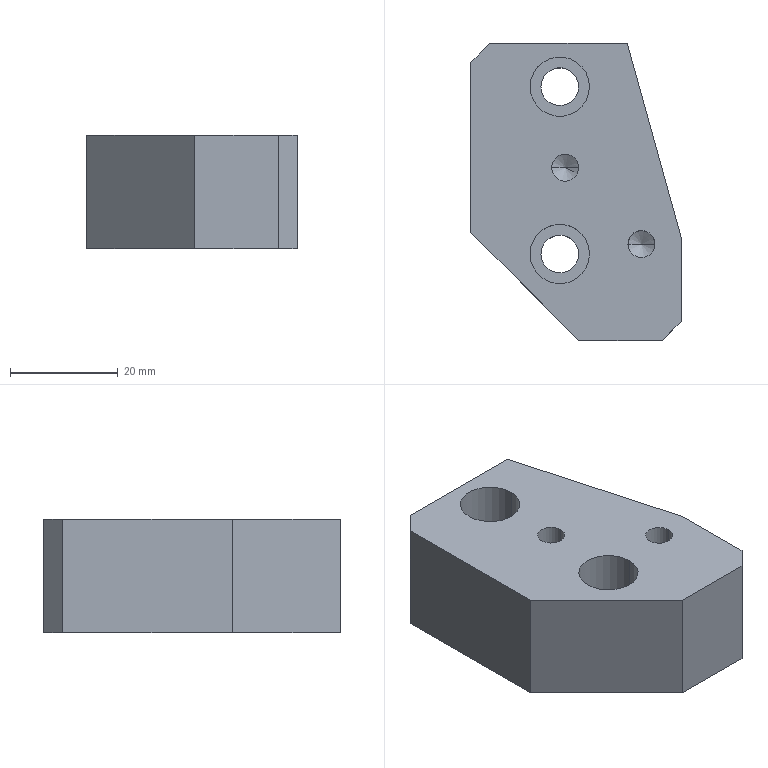Part | SolidWorks | features ICE 2, 3DProfileFeature 1, Extrusion 1, HoleWzd 1 | 1 solid | 28 faces | box 39 x 55 x 21 mm | volume 33486 mm3 | cylinder 12 | plane 12 | cone 4 | commonest cylinder face diameters 5 x4 7 x4 11 x4
STEP:
#1=CARTESIAN_POINT('',(15.,32.,4.));
#2=VERTEX_POINT('',#1);
#3=CARTESIAN_POINT('',(20.,32.,4.));
#4=VERTEX_POINT('',#3);
#5=CARTESIAN_POINT('',(17.5,32.,4.));
#6=DIRECTION('',(0.,0.,1.));
#7=DIRECTION('',(1.,0.,0.));
#8=AXIS2_PLACEMENT_3D('',#5,#6,#7);
#9=CIRCLE('',#8,2.5);
#10=EDGE_CURVE('',#2,#4,#9,.T.);
#11=ORIENTED_EDGE('',*,*,#10,.F.);
#12=CARTESIAN_POINT('',(15.,32.,21.));
#13=VERTEX_POINT('',#12);
#14=CARTESIAN_POINT('',(15.,32.,21.));
#15=DIRECTION('',(0.,0.,1.));
#16=VECTOR('',#15,1000.);
#17=LINE('',#14,#16);
#18=EDGE_CURVE('',#2,#13,#17,.T.);
#19=ORIENTED_EDGE('',*,*,#18,.T.);
#20=CARTESIAN_POINT('',(20.,32.,21.));
#21=VERTEX_POINT('',#20);
#22=CARTESIAN_POINT('',(17.5,32.,21.));
#23=DIRECTION('',(0.,0.,1.));
#24=DIRECTION('',(1.,0.,0.));
#25=AXIS2_PLACEMENT_3D('',#22,#23,#24);
#26=CIRCLE('',#25,2.5);
#27=EDGE_CURVE('',#13,#21,#26,.T.);
#28=ORIENTED_EDGE('',*,*,#27,.T.);
#29=CARTESIAN_POINT('',(20.,32.,21.));
#30=DIRECTION('',(0.,0.,1.));
#31=VECTOR('',#30,1000.);
#32=LINE('',#29,#31);
#33=EDGE_CURVE('',#4,#21,#32,.T.);
#34=ORIENTED_EDGE('',*,*,#33,.F.);
#35=EDGE_LOOP('',(#11,#19,#28,#34));
#36=FACE_OUTER_BOUND('',#35,.T.);
#37=CARTESIAN_POINT('',(17.5,32.,21.));
#38=DIRECTION('',(0.,0.,1.));
#39=DIRECTION('',(1.,0.,0.));
#40=AXIS2_PLACEMENT_3D('',#37,#38,#39);
#41=CYLINDRICAL_SURFACE('',#40,2.5);
#42=ADVANCED_FACE('',(#36),#41,.F.);
#43=CARTESIAN_POINT('',(17.5,32.,2.498));
#44=VERTEX_POINT('',#43);
#45=CARTESIAN_POINT('',(20.,32.,4.));
#46=DIRECTION('',(0.8572,0.,0.515));
#47=VECTOR('',#46,1000.);
#48=LINE('',#45,#47);
#49=EDGE_CURVE('',#44,#4,#48,.T.);
#50=ORIENTED_EDGE('',*,*,#49,.F.);
#51=CARTESIAN_POINT('',(15.,32.,4.));
#52=DIRECTION('',(-0.8572,0.,0.515));
#53=VECTOR('',#52,1000.);
#54=LINE('',#51,#53);
#55=EDGE_CURVE('',#44,#2,#54,.T.);
#56=ORIENTED_EDGE('',*,*,#55,.T.);
#57=ORIENTED_EDGE('',*,*,#10,.T.);
#58=EDGE_LOOP('',(#50,#56,#57));
#59=FACE_OUTER_BOUND('',#58,.T.);
#60=CARTESIAN_POINT('',(17.5,32.,4.));
#61=DIRECTION('',(0.,0.,1.));
#62=DIRECTION('',(1.,0.,0.));
#63=AXIS2_PLACEMENT_3D('',#60,#61,#62);
#64=CONICAL_SURFACE('',#63,2.5,1.03);
#65=ADVANCED_FACE('',(#59),#64,.F.);
#66=CARTESIAN_POINT('',(29.112,17.828,4.));
#67=VERTEX_POINT('',#66);
#68=CARTESIAN_POINT('',(34.112,17.828,4.));
#69=VERTEX_POINT('',#68);
#70=CARTESIAN_POINT('',(31.612,17.828,4.));
#71=DIRECTION('',(0.,0.,1.));
#72=DIRECTION('',(1.,0.,0.));
#73=AXIS2_PLACEMENT_3D('',#70,#71,#72);
#74=CIRCLE('',#73,2.5);
#75=EDGE_CURVE('',#67,#69,#74,.T.);
#76=ORIENTED_EDGE('',*,*,#75,.F.);
#77=CARTESIAN_POINT('',(29.112,17.828,21.));
#78=VERTEX_POINT('',#77);
#79=CARTESIAN_POINT('',(29.112,17.828,21.));
#80=DIRECTION('',(0.,0.,1.));
#81=VECTOR('',#80,1000.);
#82=LINE('',#79,#81);
#83=EDGE_CURVE('',#67,#78,#82,.T.);
#84=ORIENTED_EDGE('',*,*,#83,.T.);
#85=CARTESIAN_POINT('',(34.112,17.828,21.));
#86=VERTEX_POINT('',#85);
#87=CARTESIAN_POINT('',(31.612,17.828,21.));
#88=DIRECTION('',(0.,0.,1.));
#89=DIRECTION('',(1.,0.,0.));
#90=AXIS2_PLACEMENT_3D('',#87,#88,#89);
#91=CIRCLE('',#90,2.5);
#92=EDGE_CURVE('',#78,#86,#91,.T.);
#93=ORIENTED_EDGE('',*,*,#92,.T.);
#94=CARTESIAN_POINT('',(34.112,17.828,21.));
#95=DIRECTION('',(0.,0.,1.));
#96=VECTOR('',#95,1000.);
#97=LINE('',#94,#96);
#98=EDGE_CURVE('',#69,#86,#97,.T.);
#99=ORIENTED_EDGE('',*,*,#98,.F.);
#100=EDGE_LOOP('',(#76,#84,#93,#99));
#101=FACE_OUTER_BOUND('',#100,.T.);
#102=CARTESIAN_POINT('',(31.612,17.828,21.));
#103=DIRECTION('',(0.,0.,1.));
#104=DIRECTION('',(1.,0.,0.));
#105=AXIS2_PLACEMENT_3D('',#102,#103,#104);
#106=CYLINDRICAL_SURFACE('',#105,2.5);
#107=ADVANCED_FACE('',(#101),#106,.F.);
#108=CARTESIAN_POINT('',(31.612,17.828,2.498));
#109=VERTEX_POINT('',#108);
#110=CARTESIAN_POINT('',(34.112,17.828,4.));
#111=DIRECTION('',(0.8572,0.,0.515));
#112=VECTOR('',#111,1000.);
#113=LINE('',#110,#112);
#114=EDGE_CURVE('',#109,#69,#113,.T.);
#115=ORIENTED_EDGE('',*,*,#114,.F.);
#116=CARTESIAN_POINT('',(29.112,17.828,4.));
#117=DIRECTION('',(-0.8572,0.,0.515));
#118=VECTOR('',#117,1000.);
#119=LINE('',#116,#118);
#120=EDGE_CURVE('',#109,#67,#119,.T.);
#121=ORIENTED_EDGE('',*,*,#120,.T.);
#122=ORIENTED_EDGE('',*,*,#75,.T.);
#123=EDGE_LOOP('',(#115,#121,#122));
#124=FACE_OUTER_BOUND('',#123,.T.);
#125=CARTESIAN_POINT('',(31.612,17.828,4.));
#126=DIRECTION('',(0.,0.,1.));
#127=DIRECTION('',(1.,0.,0.));
#128=AXIS2_PLACEMENT_3D('',#125,#126,#127);
#129=CONICAL_SURFACE('',#128,2.5,1.03);
#130=ADVANCED_FACE('',(#124),#129,.F.);
#131=CARTESIAN_POINT('',(13.,16.,0.));
#132=VERTEX_POINT('',#131);
#133=CARTESIAN_POINT('',(20.,16.,0.));
#134=VERTEX_POINT('',#133);
#135=CARTESIAN_POINT('',(16.5,16.,0.));
#136=DIRECTION('',(0.,0.,1.));
#137=DIRECTION('',(1.,0.,0.));
#138=AXIS2_PLACEMENT_3D('',#135,#136,#137);
#139=CIRCLE('',#138,3.5);
#140=EDGE_CURVE('',#132,#134,#139,.T.);
#141=ORIENTED_EDGE('',*,*,#140,.F.);
#142=CARTESIAN_POINT('',(13.,16.,12.));
#143=VERTEX_POINT('',#142);
#144=CARTESIAN_POINT('',(13.,16.,0.));
#145=DIRECTION('',(0.,0.,1.));
#146=VECTOR('',#145,1000.);
#147=LINE('',#144,#146);
#148=EDGE_CURVE('',#132,#143,#147,.T.);
#149=ORIENTED_EDGE('',*,*,#148,.T.);
#150=CARTESIAN_POINT('',(20.,16.,12.));
#151=VERTEX_POINT('',#150);
#152=CARTESIAN_POINT('',(16.5,16.,12.));
#153=DIRECTION('',(0.,0.,1.));
#154=DIRECTION('',(1.,0.,0.));
#155=AXIS2_PLACEMENT_3D('',#152,#153,#154);
#156=CIRCLE('',#155,3.5);
#157=EDGE_CURVE('',#143,#151,#156,.T.);
#158=ORIENTED_EDGE('',*,*,#157,.T.);
#159=CARTESIAN_POINT('',(20.,16.,0.));
#160=DIRECTION('',(0.,0.,1.));
#161=VECTOR('',#160,1000.);
#162=LINE('',#159,#161);
#163=EDGE_CURVE('',#134,#151,#162,.T.);
#164=ORIENTED_EDGE('',*,*,#163,.F.);
#165=EDGE_LOOP('',(#141,#149,#158,#164));
#166=FACE_OUTER_BOUND('',#165,.T.);
#167=CARTESIAN_POINT('',(16.5,16.,0.));
#168=DIRECTION('',(0.,0.,1.));
#169=DIRECTION('',(1.,0.,0.));
#170=AXIS2_PLACEMENT_3D('',#167,#168,#169);
#171=CYLINDRICAL_SURFACE('',#170,3.5);
#172=ADVANCED_FACE('',(#166),#171,.F.);
#173=CARTESIAN_POINT('',(13.,47.,0.));
#174=VERTEX_POINT('',#173);
#175=CARTESIAN_POINT('',(20.,47.,0.));
#176=VERTEX_POINT('',#175);
#177=CARTESIAN_POINT('',(16.5,47.,0.));
#178=DIRECTION('',(0.,0.,1.));
#179=DIRECTION('',(1.,0.,0.));
#180=AXIS2_PLACEMENT_3D('',#177,#178,#179);
#181=CIRCLE('',#180,3.5);
#182=EDGE_CURVE('',#174,#176,#181,.T.);
#183=ORIENTED_EDGE('',*,*,#182,.F.);
#184=CARTESIAN_POINT('',(13.,47.,12.));
#185=VERTEX_POINT('',#184);
#186=CARTESIAN_POINT('',(13.,47.,0.));
#187=DIRECTION('',(0.,0.,1.));
#188=VECTOR('',#187,1000.);
#189=LINE('',#186,#188);
#190=EDGE_CURVE('',#174,#185,#189,.T.);
#191=ORIENTED_EDGE('',*,*,#190,.T.);
#192=CARTESIAN_POINT('',(20.,47.,12.));
#193=VERTEX_POINT('',#192);
#194=CARTESIAN_POINT('',(16.5,47.,12.));
#195=DIRECTION('',(0.,0.,1.));
#196=DIRECTION('',(1.,0.,0.));
#197=AXIS2_PLACEMENT_3D('',#194,#195,#196);
#198=CIRCLE('',#197,3.5);
#199=EDGE_CURVE('',#185,#193,#198,.T.);
#200=ORIENTED_EDGE('',*,*,#199,.T.);
#201=CARTESIAN_POINT('',(20.,47.,0.));
#202=DIRECTION('',(0.,0.,1.));
#203=VECTOR('',#202,1000.);
#204=LINE('',#201,#203);
#205=EDGE_CURVE('',#176,#193,#204,.T.);
#206=ORIENTED_EDGE('',*,*,#205,.F.);
#207=EDGE_LOOP('',(#183,#191,#200,#206));
#208=FACE_OUTER_BOUND('',#207,.T.);
#209=CARTESIAN_POINT('',(16.5,47.,0.));
#210=DIRECTION('',(0.,0.,1.));
#211=DIRECTION('',(1.,0.,0.));
#212=AXIS2_PLACEMENT_3D('',#209,#210,#211);
#213=CYLINDRICAL_SURFACE('',#212,3.5);
#214=ADVANCED_FACE('',(#208),#213,.F.);
#215=CARTESIAN_POINT('',(11.,16.,12.));
#216=VERTEX_POINT('',#215);
#217=CARTESIAN_POINT('',(22.,16.,12.));
#218=VERTEX_POINT('',#217);
#219=CARTESIAN_POINT('',(16.5,16.,12.));
#220=DIRECTION('',(0.,0.,1.));
#221=DIRECTION('',(1.,0.,0.));
#222=AXIS2_PLACEMENT_3D('',#219,#220,#221);
#223=CIRCLE('',#222,5.5);
#224=EDGE_CURVE('',#216,#218,#223,.T.);
#225=ORIENTED_EDGE('',*,*,#224,.F.);
#226=CARTESIAN_POINT('',(11.,16.,21.));
#227=VERTEX_POINT('',#226);
#228=CARTESIAN_POINT('',(11.,16.,12.));
#229=DIRECTION('',(0.,0.,1.));
#230=VECTOR('',#229,1000.);
#231=LINE('',#228,#230);
#232=EDGE_CURVE('',#216,#227,#231,.T.);
#233=ORIENTED_EDGE('',*,*,#232,.T.);
#234=CARTESIAN_POINT('',(22.,16.,21.));
#235=VERTEX_POINT('',#234);
#236=CARTESIAN_POINT('',(16.5,16.,21.));
#237=DIRECTION('',(0.,0.,1.));
#238=DIRECTION('',(1.,0.,0.));
#239=AXIS2_PLACEMENT_3D('',#236,#237,#238);
#240=CIRCLE('',#239,5.5);
#241=EDGE_CURVE('',#227,#235,#240,.T.);
#242=ORIENTED_EDGE('',*,*,#241,.T.);
#243=CARTESIAN_POINT('',(22.,16.,12.));
#244=DIRECTION('',(0.,0.,1.));
#245=VECTOR('',#244,1000.);
#246=LINE('',#243,#245);
#247=EDGE_CURVE('',#218,#235,#246,.T.);
#248=ORIENTED_EDGE('',*,*,#247,.F.);
#249=EDGE_LOOP('',(#225,#233,#242,#248));
#250=FACE_OUTER_BOUND('',#249,.T.);
#251=CARTESIAN_POINT('',(16.5,16.,12.));
#252=DIRECTION('',(0.,0.,1.));
#253=DIRECTION('',(1.,0.,0.));
#254=AXIS2_PLACEMENT_3D('',#251,#252,#253);
#255=CYLINDRICAL_SURFACE('',#254,5.5);
#256=ADVANCED_FACE('',(#250),#255,.F.);
#257=CARTESIAN_POINT('',(11.,47.,12.));
#258=VERTEX_POINT('',#257);
#259=CARTESIAN_POINT('',(22.,47.,12.));
#260=VERTEX_POINT('',#259);
#261=CARTESIAN_POINT('',(16.5,47.,12.));
#262=DIRECTION('',(0.,0.,1.));
#263=DIRECTION('',(1.,0.,0.));
#264=AXIS2_PLACEMENT_3D('',#261,#262,#263);
#265=CIRCLE('',#264,5.5);
#266=EDGE_CURVE('',#258,#260,#265,.T.);
#267=ORIENTED_EDGE('',*,*,#266,.F.);
#268=CARTESIAN_POINT('',(11.,47.,21.));
#269=VERTEX_POINT('',#268);
#270=CARTESIAN_POINT('',(11.,47.,12.));
#271=DIRECTION('',(0.,0.,1.));
#272=VECTOR('',#271,1000.);
#273=LINE('',#270,#272);
#274=EDGE_CURVE('',#258,#269,#273,.T.);
#275=ORIENTED_EDGE('',*,*,#274,.T.);
#276=CARTESIAN_POINT('',(22.,47.,21.));
#277=VERTEX_POINT('',#276);
#278=CARTESIAN_POINT('',(16.5,47.,21.));
#279=DIRECTION('',(0.,0.,1.));
#280=DIRECTION('',(1.,0.,0.));
#281=AXIS2_PLACEMENT_3D('',#278,#279,#280);
#282=CIRCLE('',#281,5.5);
#283=EDGE_CURVE('',#269,#277,#282,.T.);
#284=ORIENTED_EDGE('',*,*,#283,.T.);
#285=CARTESIAN_POINT('',(22.,47.,12.));
#286=DIRECTION('',(0.,0.,1.));
#287=VECTOR('',#286,1000.);
#288=LINE('',#285,#287);
#289=EDGE_CURVE('',#260,#277,#288,.T.);
#290=ORIENTED_EDGE('',*,*,#289,.F.);
#291=EDGE_LOOP('',(#267,#275,#284,#290));
#292=FACE_OUTER_BOUND('',#291,.T.);
#293=CARTESIAN_POINT('',(16.5,47.,12.));
#294=DIRECTION('',(0.,0.,1.));
#295=DIRECTION('',(1.,0.,0.));
#296=AXIS2_PLACEMENT_3D('',#293,#294,#295);
#297=CYLINDRICAL_SURFACE('',#296,5.5);
#298=ADVANCED_FACE('',(#292),#297,.F.);
#299=CARTESIAN_POINT('',(3.5,55.,0.));
#300=VERTEX_POINT('',#299);
#301=CARTESIAN_POINT('',(0.,51.5,0.));
#302=VERTEX_POINT('',#301);
#303=CARTESIAN_POINT('',(3.5,55.,0.));
#304=DIRECTION('',(-0.7071,-0.7071,0.));
#305=VECTOR('',#304,1000.);
#306=LINE('',#303,#305);
#307=EDGE_CURVE('',#300,#302,#306,.T.);
#308=ORIENTED_EDGE('',*,*,#307,.T.);
#309=CARTESIAN_POINT('',(0.,51.5,21.));
#310=VERTEX_POINT('',#309);
#311=CARTESIAN_POINT('',(0.,51.5,21.));
#312=DIRECTION('',(0.,0.,-1.));
#313=VECTOR('',#312,1000.);
#314=LINE('',#311,#313);
#315=EDGE_CURVE('',#310,#302,#314,.T.);
#316=ORIENTED_EDGE('',*,*,#315,.F.);
#317=CARTESIAN_POINT('',(3.5,55.,21.));
#318=VERTEX_POINT('',#317);
#319=CARTESIAN_POINT('',(3.5,55.,21.));
#320=DIRECTION('',(-0.7071,-0.7071,0.));
#321=VECTOR('',#320,1000.);
#322=LINE('',#319,#321);
#323=EDGE_CURVE('',#318,#310,#322,.T.);
#324=ORIENTED_EDGE('',*,*,#323,.F.);
#325=CARTESIAN_POINT('',(3.5,55.,21.));
#326=DIRECTION('',(0.,0.,-1.));
#327=VECTOR('',#326,1000.);
#328=LINE('',#325,#327);
#329=EDGE_CURVE('',#318,#300,#328,.T.);
#330=ORIENTED_EDGE('',*,*,#329,.T.);
#331=EDGE_LOOP('',(#308,#316,#324,#330));
#332=FACE_OUTER_BOUND('',#331,.T.);
#333=CARTESIAN_POINT('',(3.5,55.,21.));
#334=DIRECTION('',(0.7071,-0.7071,0.));
#335=DIRECTION('',(0.7071,0.7071,0.));
#336=AXIS2_PLACEMENT_3D('',#333,#334,#335);
#337=PLANE('',#336);
#338=ADVANCED_FACE('',(#332),#337,.F.);
#339=CARTESIAN_POINT('',(0.,20.,0.));
#340=VERTEX_POINT('',#339);
#341=CARTESIAN_POINT('',(0.,20.,0.));
#342=DIRECTION('',(0.,-1.,0.));
#343=VECTOR('',#342,1000.);
#344=LINE('',#341,#343);
#345=EDGE_CURVE('',#302,#340,#344,.T.);
#346=ORIENTED_EDGE('',*,*,#345,.T.);
#347=CARTESIAN_POINT('',(0.,20.,21.));
#348=VERTEX_POINT('',#347);
#349=CARTESIAN_POINT('',(0.,20.,21.));
#350=DIRECTION('',(0.,0.,-1.));
#351=VECTOR('',#350,1000.);
#352=LINE('',#349,#351);
#353=EDGE_CURVE('',#348,#340,#352,.T.);
#354=ORIENTED_EDGE('',*,*,#353,.F.);
#355=CARTESIAN_POINT('',(0.,20.,21.));
#356=DIRECTION('',(0.,-1.,0.));
#357=VECTOR('',#356,1000.);
#358=LINE('',#355,#357);
#359=EDGE_CURVE('',#310,#348,#358,.T.);
#360=ORIENTED_EDGE('',*,*,#359,.F.);
#361=ORIENTED_EDGE('',*,*,#315,.T.);
#362=EDGE_LOOP('',(#346,#354,#360,#361));
#363=FACE_OUTER_BOUND('',#362,.T.);
#364=CARTESIAN_POINT('',(0.,20.,21.));
#365=DIRECTION('',(1.,0.,0.));
#366=DIRECTION('',(0.,0.,-1.));
#367=AXIS2_PLACEMENT_3D('',#364,#365,#366);
#368=PLANE('',#367);
#369=ADVANCED_FACE('',(#363),#368,.F.);
#370=CARTESIAN_POINT('',(20.,0.,0.));
#371=VERTEX_POINT('',#370);
#372=CARTESIAN_POINT('',(0.,20.,0.));
#373=DIRECTION('',(0.7071,-0.7071,0.));
#374=VECTOR('',#373,1000.);
#375=LINE('',#372,#374);
#376=EDGE_CURVE('',#340,#371,#375,.T.);
#377=ORIENTED_EDGE('',*,*,#376,.T.);
#378=CARTESIAN_POINT('',(20.,0.,21.));
#379=VERTEX_POINT('',#378);
#380=CARTESIAN_POINT('',(20.,0.,21.));
#381=DIRECTION('',(0.,0.,-1.));
#382=VECTOR('',#381,1000.);
#383=LINE('',#380,#382);
#384=EDGE_CURVE('',#379,#371,#383,.T.);
#385=ORIENTED_EDGE('',*,*,#384,.F.);
#386=CARTESIAN_POINT('',(0.,20.,21.));
#387=DIRECTION('',(0.7071,-0.7071,0.));
#388=VECTOR('',#387,1000.);
#389=LINE('',#386,#388);
#390=EDGE_CURVE('',#348,#379,#389,.T.);
#391=ORIENTED_EDGE('',*,*,#390,.F.);
#392=ORIENTED_EDGE('',*,*,#353,.T.);
#393=EDGE_LOOP('',(#377,#385,#391,#392));
#394=FACE_OUTER_BOUND('',#393,.T.);
#395=CARTESIAN_POINT('',(0.,20.,21.));
#396=DIRECTION('',(0.7071,0.7071,0.));
#397=DIRECTION('',(-0.7071,0.7071,0.));
#398=AXIS2_PLACEMENT_3D('',#395,#396,#397);
#399=PLANE('',#398);
#400=ADVANCED_FACE('',(#394),#399,.F.);
#401=CARTESIAN_POINT('',(35.5,0.,0.));
#402=VERTEX_POINT('',#401);
#403=CARTESIAN_POINT('',(20.,0.,0.));
#404=DIRECTION('',(1.,0.,0.));
#405=VECTOR('',#404,1000.);
#406=LINE('',#403,#405);
#407=EDGE_CURVE('',#371,#402,#406,.T.);
#408=ORIENTED_EDGE('',*,*,#407,.T.);
#409=CARTESIAN_POINT('',(35.5,0.,21.));
#410=VERTEX_POINT('',#409);
#411=CARTESIAN_POINT('',(35.5,0.,21.));
#412=DIRECTION('',(0.,0.,-1.));
#413=VECTOR('',#412,1000.);
#414=LINE('',#411,#413);
#415=EDGE_CURVE('',#410,#402,#414,.T.);
#416=ORIENTED_EDGE('',*,*,#415,.F.);
#417=CARTESIAN_POINT('',(20.,0.,21.));
#418=DIRECTION('',(1.,0.,0.));
#419=VECTOR('',#418,1000.);
#420=LINE('',#417,#419);
#421=EDGE_CURVE('',#379,#410,#420,.T.);
#422=ORIENTED_EDGE('',*,*,#421,.F.);
#423=ORIENTED_EDGE('',*,*,#384,.T.);
#424=EDGE_LOOP('',(#408,#416,#422,#423));
#425=FACE_OUTER_BOUND('',#424,.T.);
#426=CARTESIAN_POINT('',(20.,0.,21.));
#427=DIRECTION('',(0.,1.,0.));
#428=DIRECTION('',(0.,0.,1.));
#429=AXIS2_PLACEMENT_3D('',#426,#427,#428);
#430=PLANE('',#429);
#431=ADVANCED_FACE('',(#425),#430,.F.);
#432=CARTESIAN_POINT('',(39.,3.5,0.));
#433=VERTEX_POINT('',#432);
#434=CARTESIAN_POINT('',(39.,3.5,0.));
#435=DIRECTION('',(0.7071,0.7071,0.));
#436=VECTOR('',#435,1000.);
#437=LINE('',#434,#436);
#438=EDGE_CURVE('',#402,#433,#437,.T.);
#439=ORIENTED_EDGE('',*,*,#438,.T.);
#440=CARTESIAN_POINT('',(39.,3.5,21.));
#441=VERTEX_POINT('',#440);
#442=CARTESIAN_POINT('',(39.,3.5,21.));
#443=DIRECTION('',(0.,0.,-1.));
#444=VECTOR('',#443,1000.);
#445=LINE('',#442,#444);
#446=EDGE_CURVE('',#441,#433,#445,.T.);
#447=ORIENTED_EDGE('',*,*,#446,.F.);
#448=CARTESIAN_POINT('',(39.,3.5,21.));
#449=DIRECTION('',(0.7071,0.7071,0.));
#450=VECTOR('',#449,1000.);
#451=LINE('',#448,#450);
#452=EDGE_CURVE('',#410,#441,#451,.T.);
#453=ORIENTED_EDGE('',*,*,#452,.F.);
#454=ORIENTED_EDGE('',*,*,#415,.T.);
#455=EDGE_LOOP('',(#439,#447,#453,#454));
#456=FACE_OUTER_BOUND('',#455,.T.);
#457=CARTESIAN_POINT('',(39.,3.5,21.));
#458=DIRECTION('',(-0.7071,0.7071,0.));
#459=DIRECTION('',(-0.7071,-0.7071,0.));
#460=AXIS2_PLACEMENT_3D('',#457,#458,#459);
#461=PLANE('',#460);
#462=ADVANCED_FACE('',(#456),#461,.F.);
#463=CARTESIAN_POINT('',(39.,19.,0.));
#464=VERTEX_POINT('',#463);
#465=CARTESIAN_POINT('',(39.,3.5,0.));
#466=DIRECTION('',(0.,1.,0.));
#467=VECTOR('',#466,1000.);
#468=LINE('',#465,#467);
#469=EDGE_CURVE('',#433,#464,#468,.T.);
#470=ORIENTED_EDGE('',*,*,#469,.T.);
#471=CARTESIAN_POINT('',(39.,19.,21.));
#472=VERTEX_POINT('',#471);
#473=CARTESIAN_POINT('',(39.,19.,21.));
#474=DIRECTION('',(0.,0.,-1.));
#475=VECTOR('',#474,1000.);
#476=LINE('',#473,#475);
#477=EDGE_CURVE('',#472,#464,#476,.T.);
#478=ORIENTED_EDGE('',*,*,#477,.F.);
#479=CARTESIAN_POINT('',(39.,3.5,21.));
#480=DIRECTION('',(0.,1.,0.));
#481=VECTOR('',#480,1000.);
#482=LINE('',#479,#481);
#483=EDGE_CURVE('',#441,#472,#482,.T.);
#484=ORIENTED_EDGE('',*,*,#483,.F.);
#485=ORIENTED_EDGE('',*,*,#446,.T.);
#486=EDGE_LOOP('',(#470,#478,#484,#485));
#487=FACE_OUTER_BOUND('',#486,.T.);
#488=CARTESIAN_POINT('',(39.,3.5,21.));
#489=DIRECTION('',(-1.,0.,0.));
#490=DIRECTION('',(0.,0.,1.));
#491=AXIS2_PLACEMENT_3D('',#488,#489,#490);
#492=PLANE('',#491);
#493=ADVANCED_FACE('',(#487),#492,.F.);
#494=CARTESIAN_POINT('',(29.,55.,0.));
#495=VERTEX_POINT('',#494);
#496=CARTESIAN_POINT('',(29.,55.,0.));
#497=DIRECTION('',(-0.2676,0.9635,0.));
#498=VECTOR('',#497,1000.);
#499=LINE('',#496,#498);
#500=EDGE_CURVE('',#464,#495,#499,.T.);
#501=ORIENTED_EDGE('',*,*,#500,.T.);
#502=CARTESIAN_POINT('',(29.,55.,21.));
#503=VERTEX_POINT('',#502);
#504=CARTESIAN_POINT('',(29.,55.,21.));
#505=DIRECTION('',(0.,0.,-1.));
#506=VECTOR('',#505,1000.);
#507=LINE('',#504,#506);
#508=EDGE_CURVE('',#503,#495,#507,.T.);
#509=ORIENTED_EDGE('',*,*,#508,.F.);
#510=CARTESIAN_POINT('',(29.,55.,21.));
#511=DIRECTION('',(-0.2676,0.9635,0.));
#512=VECTOR('',#511,1000.);
#513=LINE('',#510,#512);
#514=EDGE_CURVE('',#472,#503,#513,.T.);
#515=ORIENTED_EDGE('',*,*,#514,.F.);
#516=ORIENTED_EDGE('',*,*,#477,.T.);
#517=EDGE_LOOP('',(#501,#509,#515,#516));
#518=FACE_OUTER_BOUND('',#517,.T.);
#519=CARTESIAN_POINT('',(29.,55.,21.));
#520=DIRECTION('',(-0.9635,-0.2676,0.));
#521=DIRECTION('',(0.2676,-0.9635,0.));
#522=AXIS2_PLACEMENT_3D('',#519,#520,#521);
#523=PLANE('',#522);
#524=ADVANCED_FACE('',(#518),#523,.F.);
#525=CARTESIAN_POINT('',(3.5,55.,0.));
#526=DIRECTION('',(-1.,0.,0.));
#527=VECTOR('',#526,1000.);
#528=LINE('',#525,#527);
#529=EDGE_CURVE('',#495,#300,#528,.T.);
#530=ORIENTED_EDGE('',*,*,#529,.T.);
#531=ORIENTED_EDGE('',*,*,#329,.F.);
#532=CARTESIAN_POINT('',(3.5,55.,21.));
#533=DIRECTION('',(-1.,0.,0.));
#534=VECTOR('',#533,1000.);
#535=LINE('',#532,#534);
#536=EDGE_CURVE('',#503,#318,#535,.T.);
#537=ORIENTED_EDGE('',*,*,#536,.F.);
#538=ORIENTED_EDGE('',*,*,#508,.T.);
#539=EDGE_LOOP('',(#530,#531,#537,#538));
#540=FACE_OUTER_BOUND('',#539,.T.);
#541=CARTESIAN_POINT('',(3.5,55.,21.));
#542=DIRECTION('',(0.,-1.,0.));
#543=DIRECTION('',(0.,0.,-1.));
#544=AXIS2_PLACEMENT_3D('',#541,#542,#543);
#545=PLANE('',#544);
#546=ADVANCED_FACE('',(#540),#545,.F.);
#547=CARTESIAN_POINT('',(17.5,32.,21.));
#548=DIRECTION('',(0.,0.,1.));
#549=DIRECTION('',(1.,0.,0.));
#550=AXIS2_PLACEMENT_3D('',#547,#548,#549);
#551=CIRCLE('',#550,2.5);
#552=EDGE_CURVE('',#21,#13,#551,.T.);
#553=ORIENTED_EDGE('',*,*,#552,.F.);
#554=ORIENTED_EDGE('',*,*,#27,.F.);
#555=EDGE_LOOP('',(#553,#554));
#556=FACE_BOUND('',#555,.T.);
#557=CARTESIAN_POINT('',(31.612,17.828,21.));
#558=DIRECTION('',(0.,0.,1.));
#559=DIRECTION('',(1.,0.,0.));
#560=AXIS2_PLACEMENT_3D('',#557,#558,#559);
#561=CIRCLE('',#560,2.5);
#562=EDGE_CURVE('',#86,#78,#561,.T.);
#563=ORIENTED_EDGE('',*,*,#562,.F.);
#564=ORIENTED_EDGE('',*,*,#92,.F.);
#565=EDGE_LOOP('',(#563,#564));
#566=FACE_BOUND('',#565,.T.);
#567=CARTESIAN_POINT('',(16.5,16.,21.));
#568=DIRECTION('',(0.,0.,1.));
#569=DIRECTION('',(1.,0.,0.));
#570=AXIS2_PLACEMENT_3D('',#567,#568,#569);
#571=CIRCLE('',#570,5.5);
#572=EDGE_CURVE('',#235,#227,#571,.T.);
#573=ORIENTED_EDGE('',*,*,#572,.F.);
#574=ORIENTED_EDGE('',*,*,#241,.F.);
#575=EDGE_LOOP('',(#573,#574));
#576=FACE_BOUND('',#575,.T.);
#577=CARTESIAN_POINT('',(16.5,47.,21.));
#578=DIRECTION('',(0.,0.,1.));
#579=DIRECTION('',(1.,0.,0.));
#580=AXIS2_PLACEMENT_3D('',#577,#578,#579);
#581=CIRCLE('',#580,5.5);
#582=EDGE_CURVE('',#277,#269,#581,.T.);
#583=ORIENTED_EDGE('',*,*,#582,.F.);
#584=ORIENTED_EDGE('',*,*,#283,.F.);
#585=EDGE_LOOP('',(#583,#584));
#586=FACE_BOUND('',#585,.T.);
#587=ORIENTED_EDGE('',*,*,#323,.T.);
#588=ORIENTED_EDGE('',*,*,#359,.T.);
#589=ORIENTED_EDGE('',*,*,#390,.T.);
#590=ORIENTED_EDGE('',*,*,#421,.T.);
#591=ORIENTED_EDGE('',*,*,#452,.T.);
#592=ORIENTED_EDGE('',*,*,#483,.T.);
#593=ORIENTED_EDGE('',*,*,#514,.T.);
#594=ORIENTED_EDGE('',*,*,#536,.T.);
#595=EDGE_LOOP('',(#587,#588,#589,#590,#591,#592,#593,#594));
#596=FACE_OUTER_BOUND('',#595,.T.);
#597=CARTESIAN_POINT('',(0.,0.,21.));
#598=DIRECTION('',(0.,0.,1.));
#599=DIRECTION('',(1.,0.,0.));
#600=AXIS2_PLACEMENT_3D('',#597,#598,#599);
#601=PLANE('',#600);
#602=ADVANCED_FACE('',(#556,#566,#576,#586,#596),#601,.T.);
#603=CARTESIAN_POINT('',(16.5,16.,0.));
#604=DIRECTION('',(0.,0.,1.));
#605=DIRECTION('',(1.,0.,0.));
#606=AXIS2_PLACEMENT_3D('',#603,#604,#605);
#607=CIRCLE('',#606,3.5);
#608=EDGE_CURVE('',#134,#132,#607,.T.);
#609=ORIENTED_EDGE('',*,*,#608,.T.);
#610=ORIENTED_EDGE('',*,*,#140,.T.);
#611=EDGE_LOOP('',(#609,#610));
#612=FACE_BOUND('',#611,.T.);
#613=CARTESIAN_POINT('',(16.5,47.,0.));
#614=DIRECTION('',(0.,0.,1.));
#615=DIRECTION('',(1.,0.,0.));
#616=AXIS2_PLACEMENT_3D('',#613,#614,#615);
#617=CIRCLE('',#616,3.5);
#618=EDGE_CURVE('',#176,#174,#617,.T.);
#619=ORIENTED_EDGE('',*,*,#618,.T.);
#620=ORIENTED_EDGE('',*,*,#182,.T.);
#621=EDGE_LOOP('',(#619,#620));
#622=FACE_BOUND('',#621,.T.);
#623=ORIENTED_EDGE('',*,*,#307,.F.);
#624=ORIENTED_EDGE('',*,*,#529,.F.);
#625=ORIENTED_EDGE('',*,*,#500,.F.);
#626=ORIENTED_EDGE('',*,*,#469,.F.);
#627=ORIENTED_EDGE('',*,*,#438,.F.);
#628=ORIENTED_EDGE('',*,*,#407,.F.);
#629=ORIENTED_EDGE('',*,*,#376,.F.);
#630=ORIENTED_EDGE('',*,*,#345,.F.);
#631=EDGE_LOOP('',(#623,#624,#625,#626,#627,#628,#629,#630));
#632=FACE_OUTER_BOUND('',#631,.T.);
#633=CARTESIAN_POINT('',(0.,0.,0.));
#634=DIRECTION('',(0.,0.,1.));
#635=DIRECTION('',(1.,0.,0.));
#636=AXIS2_PLACEMENT_3D('',#633,#634,#635);
#637=PLANE('',#636);
#638=ADVANCED_FACE('',(#612,#622,#632),#637,.F.);
#639=ORIENTED_EDGE('',*,*,#274,.F.);
#640=CARTESIAN_POINT('',(16.5,47.,12.));
#641=DIRECTION('',(0.,0.,1.));
#642=DIRECTION('',(1.,0.,0.));
#643=AXIS2_PLACEMENT_3D('',#640,#641,#642);
#644=CIRCLE('',#643,5.5);
#645=EDGE_CURVE('',#260,#258,#644,.T.);
#646=ORIENTED_EDGE('',*,*,#645,.F.);
#647=ORIENTED_EDGE('',*,*,#289,.T.);
#648=ORIENTED_EDGE('',*,*,#582,.T.);
#649=EDGE_LOOP('',(#639,#646,#647,#648));
#650=FACE_OUTER_BOUND('',#649,.T.);
#651=CARTESIAN_POINT('',(16.5,47.,12.));
#652=DIRECTION('',(0.,0.,1.));
#653=DIRECTION('',(1.,0.,0.));
#654=AXIS2_PLACEMENT_3D('',#651,#652,#653);
#655=CYLINDRICAL_SURFACE('',#654,5.5);
#656=ADVANCED_FACE('',(#650),#655,.F.);
#657=CARTESIAN_POINT('',(16.5,47.,12.));
#658=DIRECTION('',(0.,0.,1.));
#659=DIRECTION('',(1.,0.,0.));
#660=AXIS2_PLACEMENT_3D('',#657,#658,#659);
#661=CIRCLE('',#660,3.5);
#662=EDGE_CURVE('',#193,#185,#661,.T.);
#663=ORIENTED_EDGE('',*,*,#662,.F.);
#664=ORIENTED_EDGE('',*,*,#199,.F.);
#665=EDGE_LOOP('',(#663,#664));
#666=FACE_BOUND('',#665,.T.);
#667=ORIENTED_EDGE('',*,*,#645,.T.);
#668=ORIENTED_EDGE('',*,*,#266,.T.);
#669=EDGE_LOOP('',(#667,#668));
#670=FACE_OUTER_BOUND('',#669,.T.);
#671=CARTESIAN_POINT('',(16.5,47.,12.));
#672=DIRECTION('',(0.,0.,1.));
#673=DIRECTION('',(1.,0.,0.));
#674=AXIS2_PLACEMENT_3D('',#671,#672,#673);
#675=PLANE('',#674);
#676=ADVANCED_FACE('',(#666,#670),#675,.T.);
#677=ORIENTED_EDGE('',*,*,#232,.F.);
#678=CARTESIAN_POINT('',(16.5,16.,12.));
#679=DIRECTION('',(0.,0.,1.));
#680=DIRECTION('',(1.,0.,0.));
#681=AXIS2_PLACEMENT_3D('',#678,#679,#680);
#682=CIRCLE('',#681,5.5);
#683=EDGE_CURVE('',#218,#216,#682,.T.);
#684=ORIENTED_EDGE('',*,*,#683,.F.);
#685=ORIENTED_EDGE('',*,*,#247,.T.);
#686=ORIENTED_EDGE('',*,*,#572,.T.);
#687=EDGE_LOOP('',(#677,#684,#685,#686));
#688=FACE_OUTER_BOUND('',#687,.T.);
#689=CARTESIAN_POINT('',(16.5,16.,12.));
#690=DIRECTION('',(0.,0.,1.));
#691=DIRECTION('',(1.,0.,0.));
#692=AXIS2_PLACEMENT_3D('',#689,#690,#691);
#693=CYLINDRICAL_SURFACE('',#692,5.5);
#694=ADVANCED_FACE('',(#688),#693,.F.);
#695=CARTESIAN_POINT('',(16.5,16.,12.));
#696=DIRECTION('',(0.,0.,1.));
#697=DIRECTION('',(1.,0.,0.));
#698=AXIS2_PLACEMENT_3D('',#695,#696,#697);
#699=CIRCLE('',#698,3.5);
#700=EDGE_CURVE('',#151,#143,#699,.T.);
#701=ORIENTED_EDGE('',*,*,#700,.F.);
#702=ORIENTED_EDGE('',*,*,#157,.F.);
#703=EDGE_LOOP('',(#701,#702));
#704=FACE_BOUND('',#703,.T.);
#705=ORIENTED_EDGE('',*,*,#683,.T.);
#706=ORIENTED_EDGE('',*,*,#224,.T.);
#707=EDGE_LOOP('',(#705,#706));
#708=FACE_OUTER_BOUND('',#707,.T.);
#709=CARTESIAN_POINT('',(16.5,16.,12.));
#710=DIRECTION('',(0.,0.,1.));
#711=DIRECTION('',(1.,0.,0.));
#712=AXIS2_PLACEMENT_3D('',#709,#710,#711);
#713=PLANE('',#712);
#714=ADVANCED_FACE('',(#704,#708),#713,.T.);
#715=ORIENTED_EDGE('',*,*,#190,.F.);
#716=ORIENTED_EDGE('',*,*,#618,.F.);
#717=ORIENTED_EDGE('',*,*,#205,.T.);
#718=ORIENTED_EDGE('',*,*,#662,.T.);
#719=EDGE_LOOP('',(#715,#716,#717,#718));
#720=FACE_OUTER_BOUND('',#719,.T.);
#721=CARTESIAN_POINT('',(16.5,47.,0.));
#722=DIRECTION('',(0.,0.,1.));
#723=DIRECTION('',(1.,0.,0.));
#724=AXIS2_PLACEMENT_3D('',#721,#722,#723);
#725=CYLINDRICAL_SURFACE('',#724,3.5);
#726=ADVANCED_FACE('',(#720),#725,.F.);
#727=ORIENTED_EDGE('',*,*,#148,.F.);
#728=ORIENTED_EDGE('',*,*,#608,.F.);
#729=ORIENTED_EDGE('',*,*,#163,.T.);
#730=ORIENTED_EDGE('',*,*,#700,.T.);
#731=EDGE_LOOP('',(#727,#728,#729,#730));
#732=FACE_OUTER_BOUND('',#731,.T.);
#733=CARTESIAN_POINT('',(16.5,16.,0.));
#734=DIRECTION('',(0.,0.,1.));
#735=DIRECTION('',(1.,0.,0.));
#736=AXIS2_PLACEMENT_3D('',#733,#734,#735);
#737=CYLINDRICAL_SURFACE('',#736,3.5);
#738=ADVANCED_FACE('',(#732),#737,.F.);
#739=ORIENTED_EDGE('',*,*,#120,.F.);
#740=ORIENTED_EDGE('',*,*,#114,.T.);
#741=CARTESIAN_POINT('',(31.612,17.828,4.));
#742=DIRECTION('',(0.,0.,1.));
#743=DIRECTION('',(1.,0.,0.));
#744=AXIS2_PLACEMENT_3D('',#741,#742,#743);
#745=CIRCLE('',#744,2.5);
#746=EDGE_CURVE('',#69,#67,#745,.T.);
#747=ORIENTED_EDGE('',*,*,#746,.T.);
#748=EDGE_LOOP('',(#739,#740,#747));
#749=FACE_OUTER_BOUND('',#748,.T.);
#750=CARTESIAN_POINT('',(31.612,17.828,4.));
#751=DIRECTION('',(0.,0.,1.));
#752=DIRECTION('',(1.,0.,0.));
#753=AXIS2_PLACEMENT_3D('',#750,#751,#752);
#754=CONICAL_SURFACE('',#753,2.5,1.03);
#755=ADVANCED_FACE('',(#749),#754,.F.);
#756=ORIENTED_EDGE('',*,*,#83,.F.);
#757=ORIENTED_EDGE('',*,*,#746,.F.);
#758=ORIENTED_EDGE('',*,*,#98,.T.);
#759=ORIENTED_EDGE('',*,*,#562,.T.);
#760=EDGE_LOOP('',(#756,#757,#758,#759));
#761=FACE_OUTER_BOUND('',#760,.T.);
#762=CARTESIAN_POINT('',(31.612,17.828,21.));
#763=DIRECTION('',(0.,0.,1.));
#764=DIRECTION('',(1.,0.,0.));
#765=AXIS2_PLACEMENT_3D('',#762,#763,#764);
#766=CYLINDRICAL_SURFACE('',#765,2.5);
#767=ADVANCED_FACE('',(#761),#766,.F.);
#768=ORIENTED_EDGE('',*,*,#55,.F.);
#769=ORIENTED_EDGE('',*,*,#49,.T.);
#770=CARTESIAN_POINT('',(17.5,32.,4.));
#771=DIRECTION('',(0.,0.,1.));
#772=DIRECTION('',(1.,0.,0.));
#773=AXIS2_PLACEMENT_3D('',#770,#771,#772);
#774=CIRCLE('',#773,2.5);
#775=EDGE_CURVE('',#4,#2,#774,.T.);
#776=ORIENTED_EDGE('',*,*,#775,.T.);
#777=EDGE_LOOP('',(#768,#769,#776));
#778=FACE_OUTER_BOUND('',#777,.T.);
#779=CARTESIAN_POINT('',(17.5,32.,4.));
#780=DIRECTION('',(0.,0.,1.));
#781=DIRECTION('',(1.,0.,0.));
#782=AXIS2_PLACEMENT_3D('',#779,#780,#781);
#783=CONICAL_SURFACE('',#782,2.5,1.03);
#784=ADVANCED_FACE('',(#778),#783,.F.);
#785=ORIENTED_EDGE('',*,*,#18,.F.);
#786=ORIENTED_EDGE('',*,*,#775,.F.);
#787=ORIENTED_EDGE('',*,*,#33,.T.);
#788=ORIENTED_EDGE('',*,*,#552,.T.);
#789=EDGE_LOOP('',(#785,#786,#787,#788));
#790=FACE_OUTER_BOUND('',#789,.T.);
#791=CARTESIAN_POINT('',(17.5,32.,21.));
#792=DIRECTION('',(0.,0.,1.));
#793=DIRECTION('',(1.,0.,0.));
#794=AXIS2_PLACEMENT_3D('',#791,#792,#793);
#795=CYLINDRICAL_SURFACE('',#794,2.5);
#796=ADVANCED_FACE('',(#790),#795,.F.);
#797=CLOSED_SHELL('',(#42,#65,#107,#130,#172,#214,#256,#298,#338,#369,#400,#431,#462,#493,#524,#546,#602,#638,#656,#676,#694,#714,#726,#738,#755,#767,#784,#796));
#798=MANIFOLD_SOLID_BREP('',#797);
#799=CARTESIAN_POINT('',(0.,0.,0.));
#800=DIRECTION('',(0.,0.,1.));
#801=DIRECTION('',(1.,0.,0.));
#802=AXIS2_PLACEMENT_3D('',#799,#800,#801);
#803=(LENGTH_UNIT()NAMED_UNIT(*)SI_UNIT(.MILLI.,.METRE.));
#804=UNCERTAINTY_MEASURE_WITH_UNIT(LENGTH_MEASURE(0.00001),#803,'','');
#805=(NAMED_UNIT(*)PLANE_ANGLE_UNIT()SI_UNIT($,.RADIAN.));
#806=(NAMED_UNIT(*)SI_UNIT($,.STERADIAN.)SOLID_ANGLE_UNIT());
#807=(GEOMETRIC_REPRESENTATION_CONTEXT(3)GLOBAL_UNCERTAINTY_ASSIGNED_CONTEXT((#804))GLOBAL_UNIT_ASSIGNED_CONTEXT((#803,#805,#806))REPRESENTATION_CONTEXT('',''));
#808=ADVANCED_BREP_SHAPE_REPRESENTATION('',(#798,#802),#807);